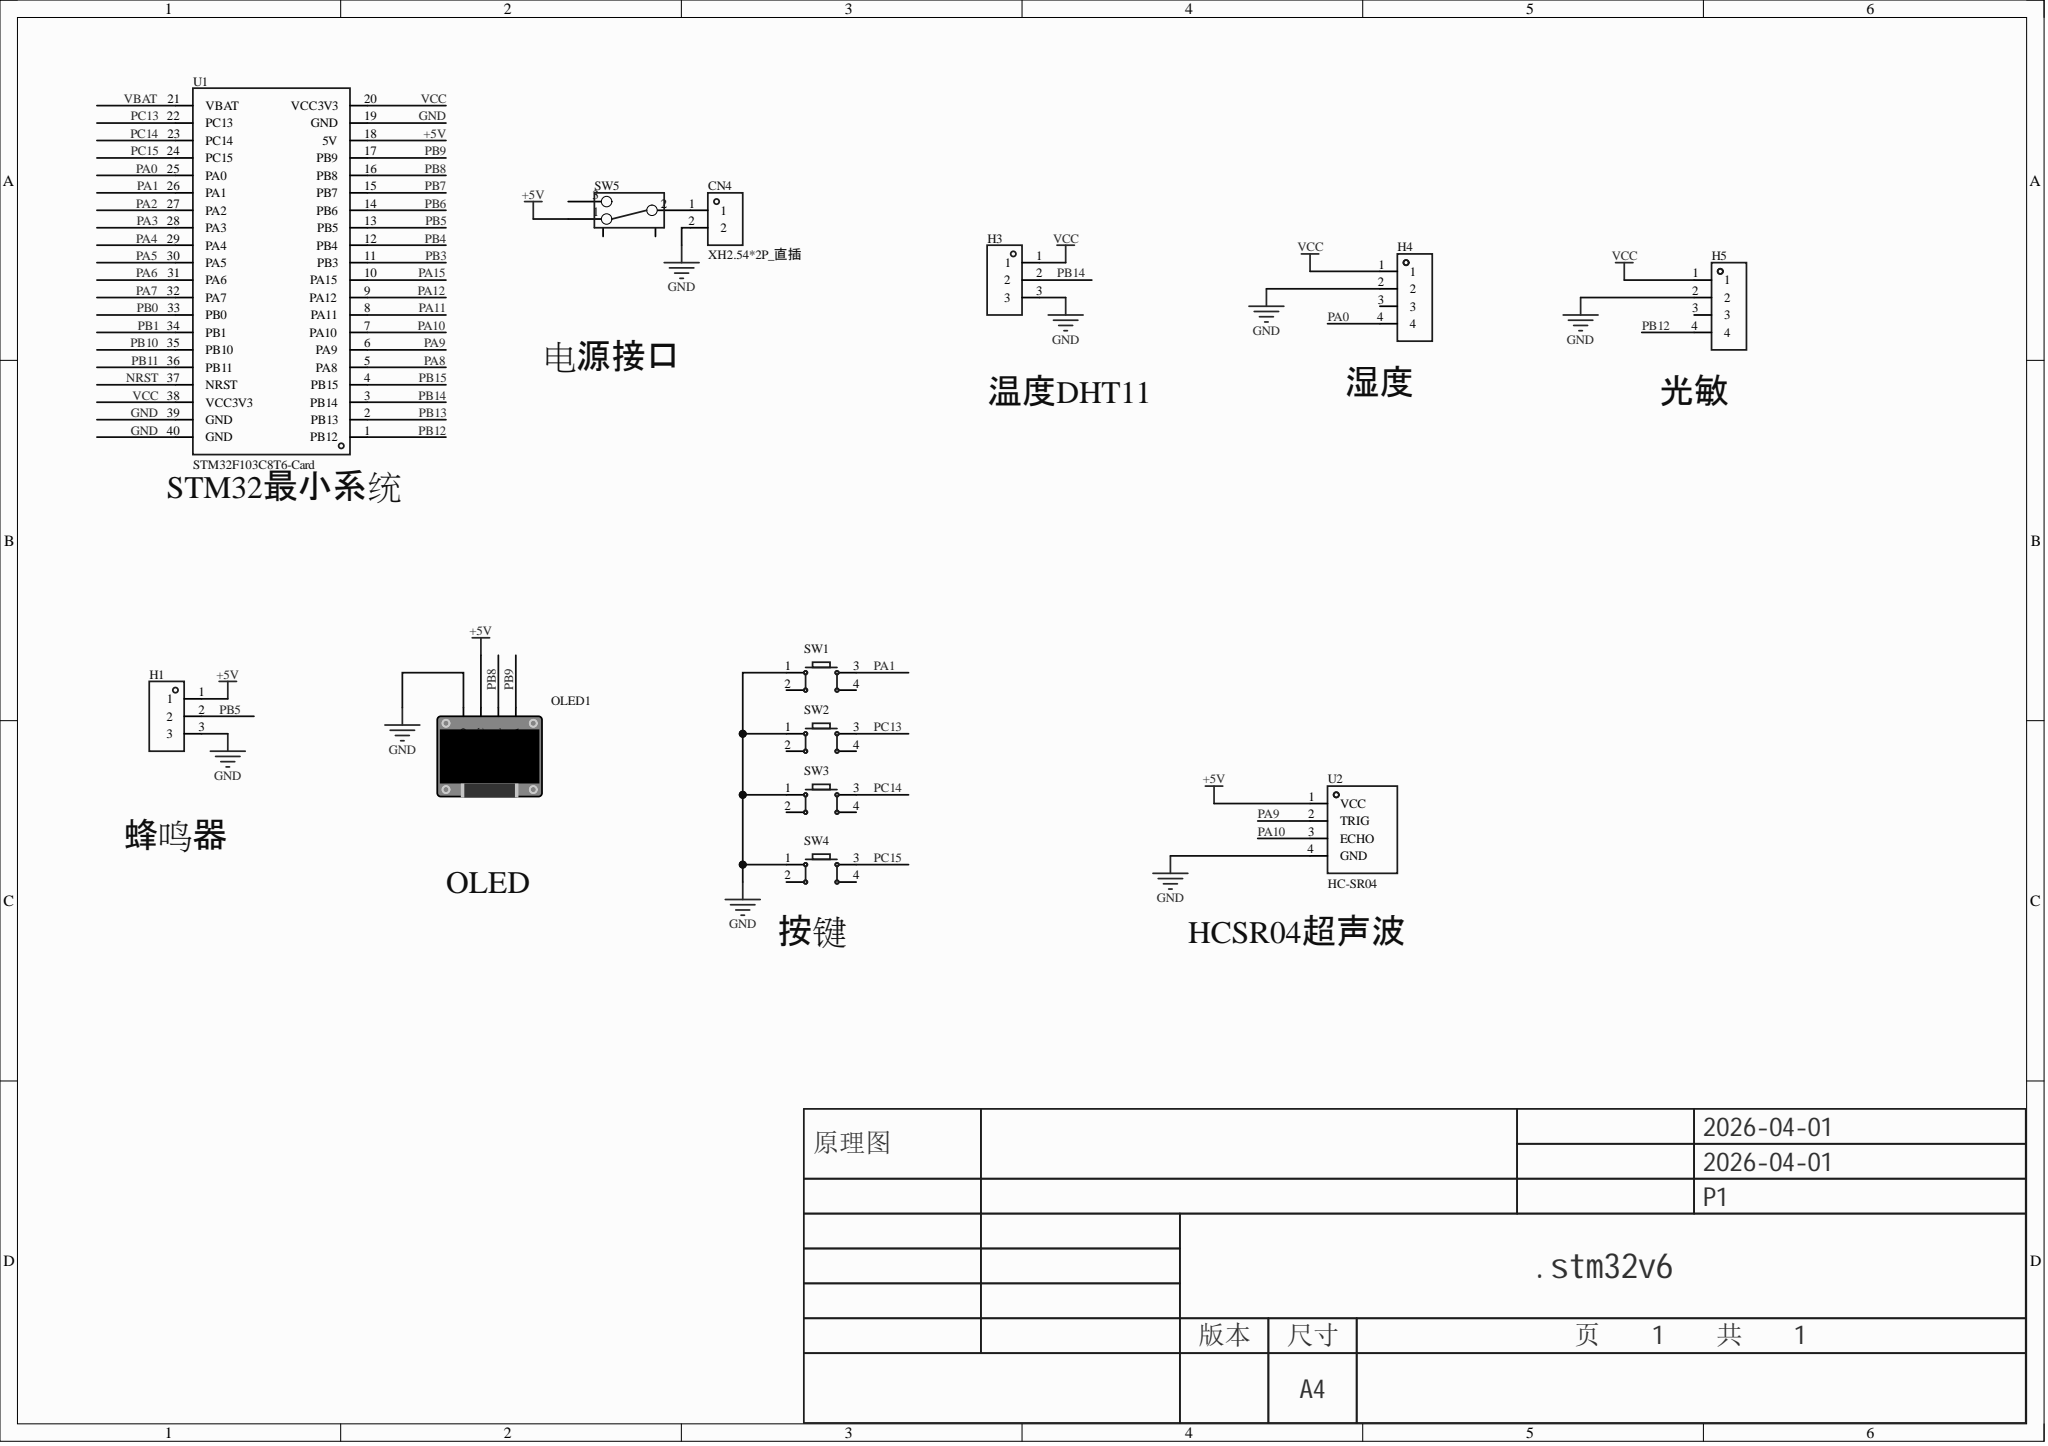Circuit board | Altium Designer | 13 parts | 16 nets
Bill of materials:
Comment,Description,Designator,Footprint,LibRef,Quantity
"XH2.54*2P_直插","","CN4","CONN-TH_2P-P2.50-XH2.54-2P","XH2.54*2P_直插","1"
"","","H1, H3","HDR-TH_3P-P2.54-V-F","HDR-F_2.54_1x3P","2"
"","","H4, H5","HDR-TH_4P-P2.54-V-F","HDR-F_2.54_1x4P","2"
"","","OLED1","0.96OLED_4P","0.96OLED模块_4P","1"
"","","SW1, SW2, SW3, SW4","SW-TH_4P-L6.0-W6.0-P4.50-LS6.5","Key_TH_6x6x6","4"
"","","SW5","拨动开关","拨动开关_正","1"
"STM32F103C8T6-Card","","U1","CONN-TH_L53.3-W22.9_STM32F103C8T6-CARD","STM32F103C8T6-Card","1"
"HC-SR04","","U2","TH_HC-SR04V","HC-SR04","1"
Netlist (Protel format):
[
CN4
CONN-TH_2P-P2.50-XH2.54-2P
XH2.54*2P_直插



]
[
H1
HDR-TH_3P-P2.54-V-F




]
[
H3
HDR-TH_3P-P2.54-V-F




]
[
H4
HDR-TH_4P-P2.54-V-F




]
[
H5
HDR-TH_4P-P2.54-V-F




]
[
OLED1
0.96OLED_4P




]
[
SW1
SW-TH_4P-L6.0-W6.0-P4.50-LS6.5




]
[
SW2
SW-TH_4P-L6.0-W6.0-P4.50-LS6.5




]
[
SW3
SW-TH_4P-L6.0-W6.0-P4.50-LS6.5




]
[
SW4
SW-TH_4P-L6.0-W6.0-P4.50-LS6.5




]
[
SW5
拨动开关




]
[
U1
CONN-TH_L53.3-W22.9_STM32F103C8T6-CARD
STM32F103C8T6-Card



]
[
U2
TH_HC-SR04V
HC-SR04



]
(
VCC
H3-1
H4-1
H5-1
U1-20
U1-38
)
(
PC15
SW4-3
U1-24
)
(
PC14
SW3-3
U1-23
)
(
PC13
SW2-3
U1-22
)
(
PB14
H3-2
U1-3
)
(
PB12
H5-4
U1-1
)
(
PB9
OLED1-4
U1-17
)
(
PB8
OLED1-3
U1-16
)
(
PB5
H1-2
U1-13
)
(
PA10
U1-7
U2-3
)
(
PA9
U1-6
U2-2
)
(
PA1
SW1-3
U1-26
)
(
PA0
H4-4
U1-25
)
(
NetCN4_1
CN4-1
SW5-2
)
(
GND
CN4-2
H1-3
H3-3
H4-2
H5-2
OLED1-1
SW1-1
SW2-1
SW3-1
SW4-1
U1-19
U1-39
U1-40
U2-4
)
(
+5V
H1-1
OLED1-2
SW5-1
U1-18
U2-1
)